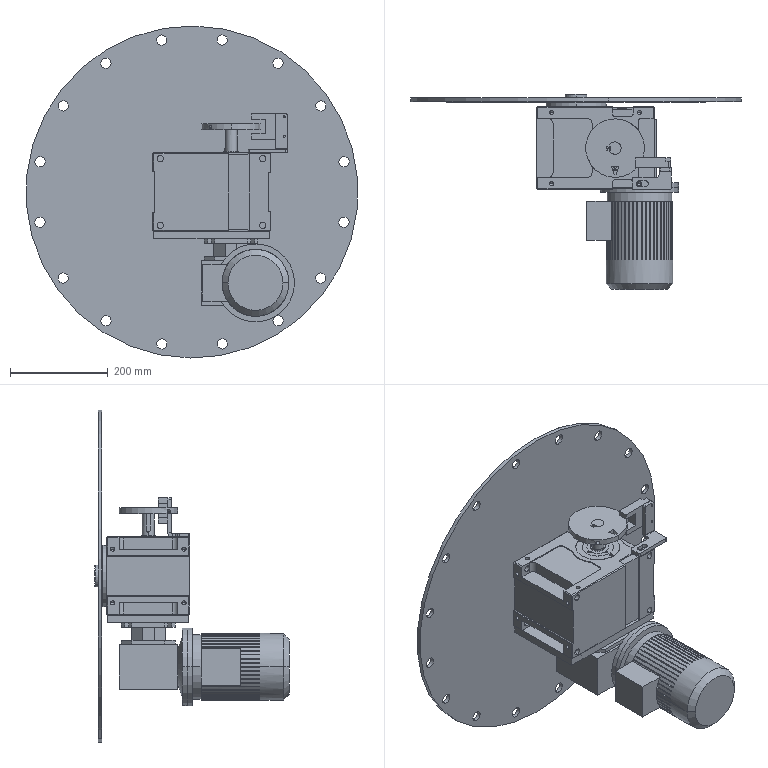Part | 10 solids | 965 faces | box 680 x 399 x 680 mm | volume 15191449 mm3 | plane 494 | cylinder 258 | spline 139 | cone 74 | commonest cylinder face diameters 8.5 x32 21 x32 8 x18 4.7 x16 13 x16 11 x14